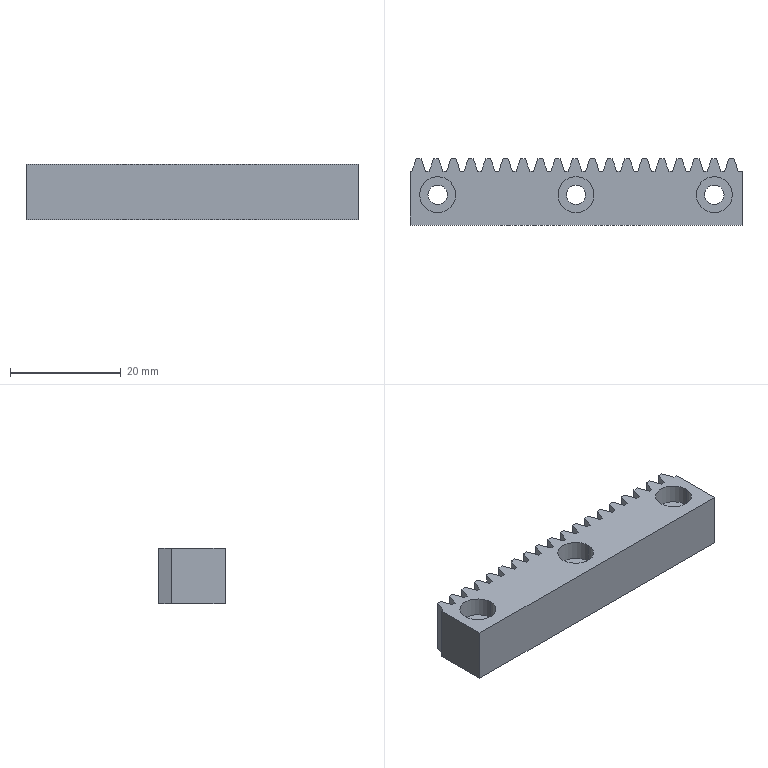Part | SolidWorks | features BaseBody 1 | 1 solid | 98 faces | box 60 x 12 x 10 mm | volume 6024 mm3 | plane 86 | cylinder 12 | commonest cylinder face diameters 3.5 x6 6.5 x6